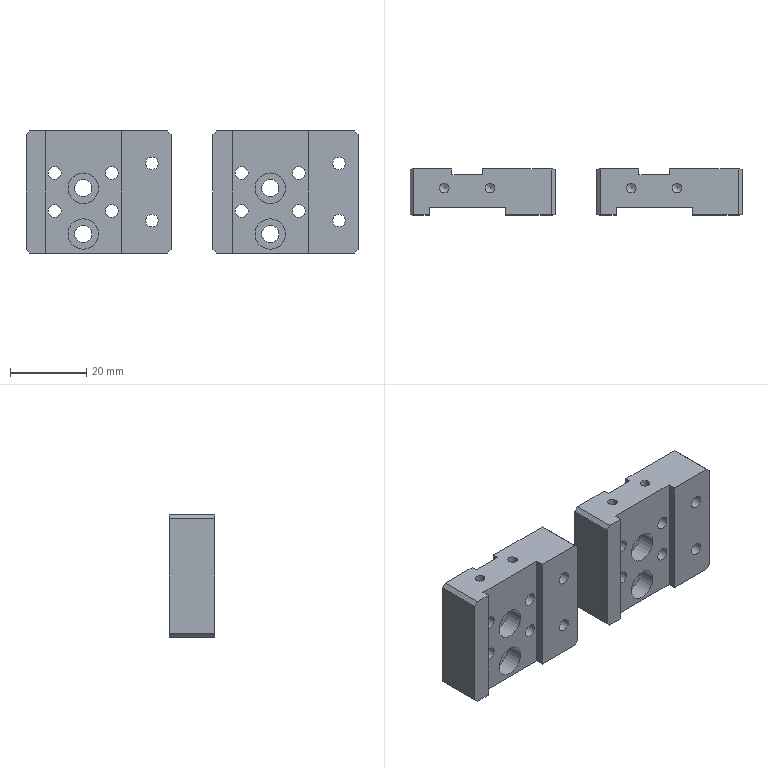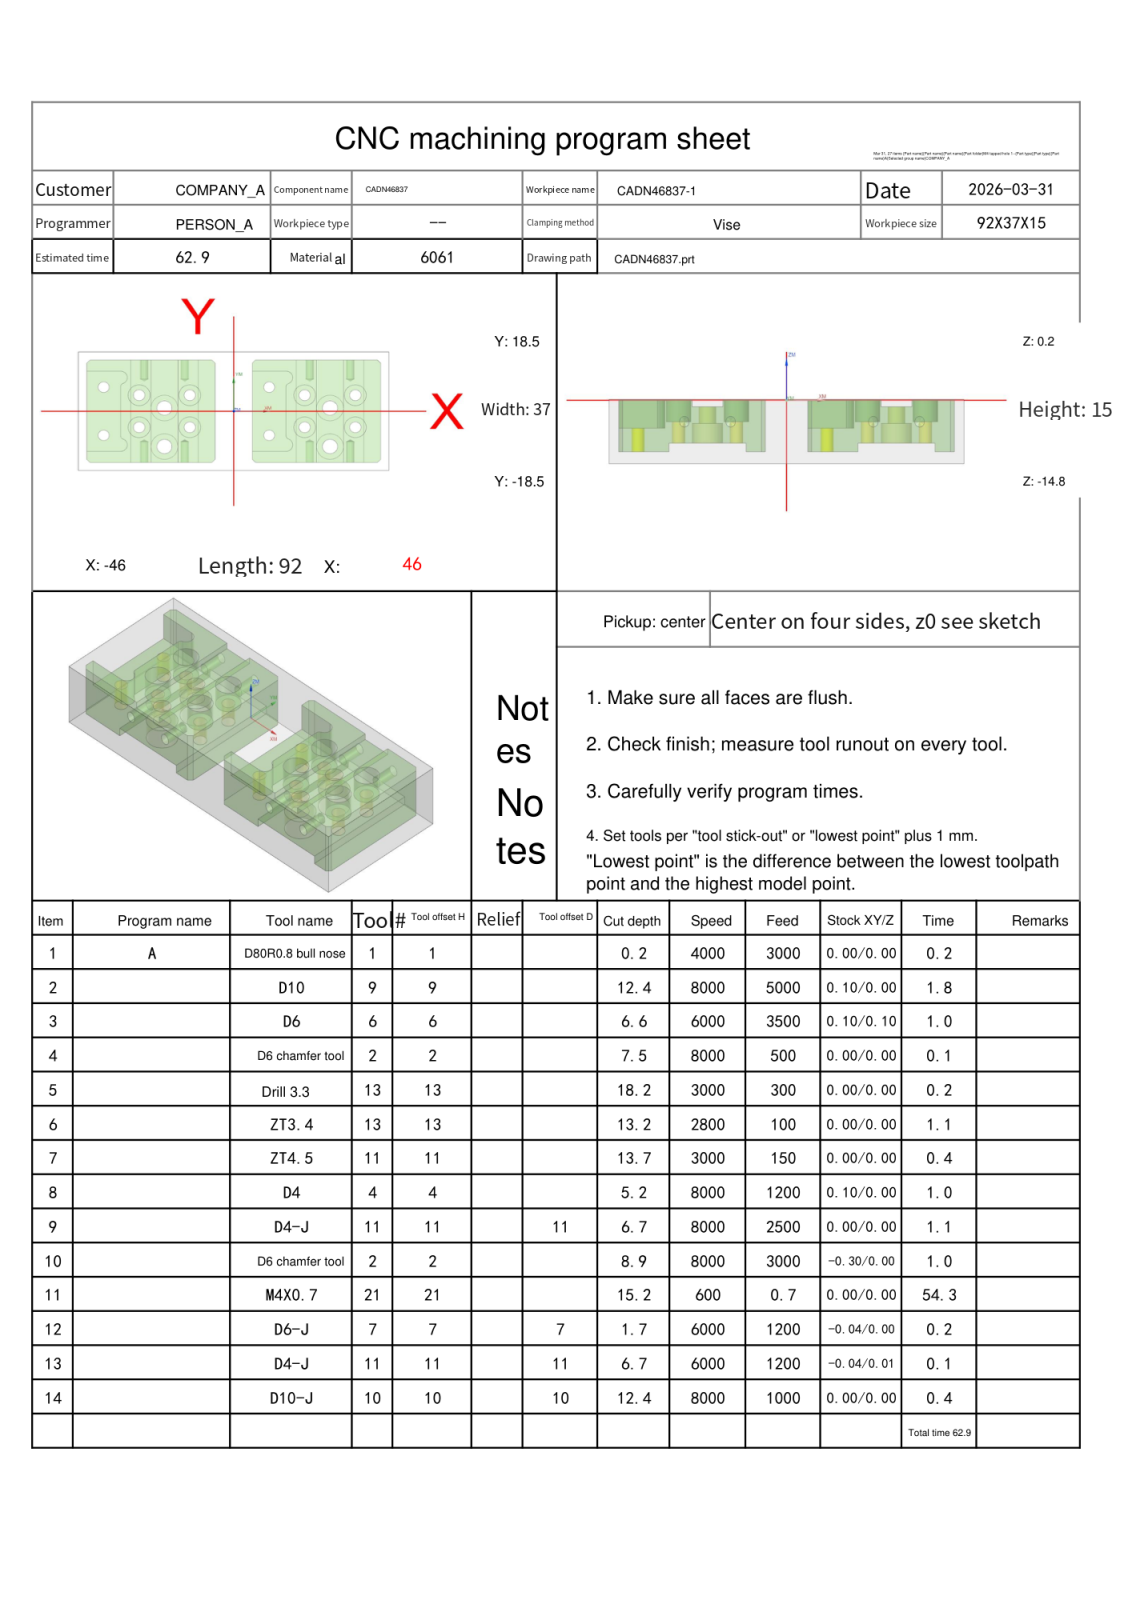NC program | NX | posted by the shop | part box 87 x 12 x 32 mm
Lines 1 to 2025 of 5636, first 1616 of 2023 lines:
%
O0001
(Machine time: 114.10 MIN)
(===Total Tool:10===)
(T1=D80R0.8 bull nose D=80.  R=0.8  D-  H01 Z=0.    )
(T9=D10     D=10.  R=0.   D-  H09 Z=-12.2 )
(T6=D6      D=6.   R=0.   D-  H06 Z=-6.4  )
(T2=D6 chamfer tool   D=6.   R=0.   D-  H02 Z=-8.7  )
(T13=Drill 3.3  D=3.3  DR_a=118 D-  H13 Z=-17.99)
(T11=ZT4.5  D=4.5  DR_a=118 D-  H11 Z=-13.5 )
(T4=D4      D=4.   R=0.   D-  H04 Z=-5.   )
(T21=M4X0.7 D=3.3  DR_a=180 D-  H21 Z=-15.  )
(T7=D6-J    D=6.   R=0.   D7  H07 Z=-1.5  )
(T10=D10-J  D=10.  R=0.   D10 H10 Z=-12.2 )
G80 G90 G17 G49 G40
G91 G28 Z0
M01
N1 T01 M06
(D80R0.8 bull nose  D=80. R=0.8 H=01 ce=0.20 di=0.10)
G00 G90 G54 X-88.5 Y0.0 M03 S4000
G43 H01 Z20.
M08
Z2.1
G01 Z.1 F3000.
X-83.5
X83.5
X88.5
Z2.1
G00 Z20.
G00 G90 X-88.5 Y0.0 M03 S4000
Z20.
Z2.
G01 Z0.0 F1000.
X-83.5
X83.5
X88.5
Z2.
G00 Z20.
G91 G28 Z0.0
M05
M09
G91 G28 Z0.0
M01
N2 T09 M06
(D10  D=10. R=0. H=09 ce=0.10 di=0.00)
G00 G90 G54 X24.5 Y-21.1 M03 S8000
G43 H09 Z20.
M08
Z.5
G01 X6.5 Z.448 F5000.
G02 X2.894 Y-19.606 Z.437 I0.0 J5.1
G01 X1.894 Y-18.606 Z.433
G02 X.4 Y-15. Z.421 I3.606 J3.606
G01 Y15. Z.335
G02 X1.894 Y18.606 Z.323 I5.1 J0.0
G01 X2.894 Y19.606 Z.319
G02 X6.5 Y21.1 Z.308 I3.606 J-3.606
G01 X42.5 Z.204
G02 X46.106 Y19.606 Z.192 I0.0 J-5.1
G01 X47.106 Y18.606 Z.188
G02 X48.6 Y15. Z.177 I-3.606 J-3.606
G01 Y-15. Z.09
G02 X47.106 Y-18.606 Z.079 I-5.1 J0.0
G01 X46.106 Y-19.606 Z.075
G02 X44.375 Y-20.743 Z.069 I-3.606 J3.606
X42.5 Y-21.1 Z.063 I-1.875 J4.743
G01 X6.5 Z-.04
G02 X2.894 Y-19.606 Z-.052 I0.0 J5.1
G01 X1.894 Y-18.606 Z-.056
G02 X.4 Y-15. Z-.067 I3.606 J3.606
G01 Y15. Z-.154
G02 X1.894 Y18.606 Z-.165 I5.1 J0.0
G01 X2.894 Y19.606 Z-.169
G02 X6.5 Y21.1 Z-.181 I3.606 J-3.606
G01 X42.5 Z-.285
G02 X46.106 Y19.606 Z-.296 I0.0 J-5.1
G01 X47.106 Y18.606 Z-.3
G02 X48.6 Y15. Z-.312 I-3.606 J-3.606
G01 Y-15. Z-.398
G02 X47.106 Y-18.606 Z-.41 I-5.1 J0.0
G01 X46.106 Y-19.606 Z-.414
G02 X44.375 Y-20.743 Z-.42 I-3.606 J3.606
X42.5 Y-21.1 Z-.425 I-1.875 J4.743
G01 X6.5 Z-.529
G02 X2.894 Y-19.606 Z-.54 I0.0 J5.1
G01 X1.894 Y-18.606 Z-.544
G02 X.4 Y-15. Z-.556 I3.606 J3.606
G01 Y15. Z-.642
G02 X1.894 Y18.606 Z-.654 I5.1 J0.0
G01 X2.894 Y19.606 Z-.658
G02 X6.5 Y21.1 Z-.669 I3.606 J-3.606
G01 X42.5 Z-.773
G02 X46.106 Y19.606 Z-.784 I0.0 J-5.1
G01 X47.106 Y18.606 Z-.789
G02 X48.6 Y15. Z-.8 I-3.606 J-3.606
G01 Y-15. Z-.886
G02 X47.106 Y-18.606 Z-.898 I-5.1 J0.0
G01 X46.106 Y-19.606 Z-.902
G02 X44.375 Y-20.743 Z-.908 I-3.606 J3.606
X42.5 Y-21.1 Z-.914 I-1.875 J4.743
G01 X6.5 Z-1.017
G02 X2.894 Y-19.606 Z-1.029 I0.0 J5.1
G01 X1.894 Y-18.606 Z-1.033
G02 X.4 Y-15. Z-1.044 I3.606 J3.606
G01 Y15. Z-1.131
G02 X1.894 Y18.606 Z-1.142 I5.1 J0.0
G01 X2.894 Y19.606 Z-1.146
G02 X6.5 Y21.1 Z-1.158 I3.606 J-3.606
G01 X42.5 Z-1.261
G02 X46.106 Y19.606 Z-1.273 I0.0 J-5.1
G01 X47.106 Y18.606 Z-1.277
G02 X48.6 Y15. Z-1.289 I-3.606 J-3.606
G01 Y-15. Z-1.375
G02 X47.106 Y-18.606 Z-1.386 I-5.1 J0.0
G01 X46.106 Y-19.606 Z-1.391
G02 X44.375 Y-20.743 Z-1.397 I-3.606 J3.606
X42.5 Y-21.1 Z-1.402 I-1.875 J4.743
G01 X6.5 Z-1.506
G02 X2.894 Y-19.606 Z-1.517 I0.0 J5.1
G01 X1.894 Y-18.606 Z-1.521
G02 X.4 Y-15. Z-1.533 I3.606 J3.606
G01 Y15. Z-1.619
G02 X1.894 Y18.606 Z-1.631 I5.1 J0.0
G01 X2.894 Y19.606 Z-1.635
G02 X6.5 Y21.1 Z-1.646 I3.606 J-3.606
G01 X42.5 Z-1.75
G02 X46.106 Y19.606 Z-1.761 I0.0 J-5.1
G01 X47.106 Y18.606 Z-1.765
G02 X48.6 Y15. Z-1.777 I-3.606 J-3.606
G01 Y-15. Z-1.863
G02 X47.106 Y-18.606 Z-1.875 I-5.1 J0.0
G01 X46.106 Y-19.606 Z-1.879
G02 X44.375 Y-20.743 Z-1.885 I-3.606 J3.606
X42.5 Y-21.1 Z-1.89 I-1.875 J4.743
G01 X6.5 Z-1.994
G02 X2.894 Y-19.606 Z-2.006 I0.0 J5.1
G01 X1.894 Y-18.606 Z-2.01
G02 X.4 Y-15. Z-2.021 I3.606 J3.606
G01 Y15. Z-2.108
G02 X1.894 Y18.606 Z-2.119 I5.1 J0.0
G01 X2.894 Y19.606 Z-2.123
G02 X6.5 Y21.1 Z-2.135 I3.606 J-3.606
G01 X42.5 Z-2.238
G02 X46.106 Y19.606 Z-2.25 I0.0 J-5.1
G01 X47.106 Y18.606 Z-2.254
G02 X48.6 Y15. Z-2.265 I-3.606 J-3.606
G01 Y-15. Z-2.352
G02 X47.106 Y-18.606 Z-2.363 I-5.1 J0.0
G01 X46.106 Y-19.606 Z-2.367
G02 X44.375 Y-20.743 Z-2.373 I-3.606 J3.606
X42.5 Y-21.1 Z-2.379 I-1.875 J4.743
G01 X6.5 Z-2.483
G02 X2.894 Y-19.606 Z-2.494 I0.0 J5.1
G01 X1.894 Y-18.606 Z-2.498
G02 X.4 Y-15. Z-2.51 I3.606 J3.606
G01 Y15. Z-2.596
G02 X1.894 Y18.606 Z-2.608 I5.1 J0.0
G01 X2.894 Y19.606 Z-2.612
G02 X6.5 Y21.1 Z-2.623 I3.606 J-3.606
G01 X42.5 Z-2.727
G02 X46.106 Y19.606 Z-2.738 I0.0 J-5.1
G01 X47.106 Y18.606 Z-2.742
G02 X48.6 Y15. Z-2.754 I-3.606 J-3.606
G01 Y-15. Z-2.84
G02 X47.106 Y-18.606 Z-2.852 I-5.1 J0.0
G01 X46.106 Y-19.606 Z-2.856
G02 X44.375 Y-20.743 Z-2.862 I-3.606 J3.606
X42.5 Y-21.1 Z-2.867 I-1.875 J4.743
G01 X6.5 Z-2.971
G02 X2.894 Y-19.606 Z-2.983 I0.0 J5.1
G01 X1.894 Y-18.606 Z-2.987
G02 X.4 Y-15. Z-2.998 I3.606 J3.606
G01 Y15. Z-3.085
G02 X1.894 Y18.606 Z-3.096 I5.1 J0.0
G01 X2.894 Y19.606 Z-3.1
G02 X6.5 Y21.1 Z-3.112 I3.606 J-3.606
G01 X42.5 Z-3.215
G02 X46.106 Y19.606 Z-3.227 I0.0 J-5.1
G01 X47.106 Y18.606 Z-3.231
G02 X48.6 Y15. Z-3.242 I-3.606 J-3.606
G01 Y-15. Z-3.329
G02 X47.106 Y-18.606 Z-3.34 I-5.1 J0.0
G01 X46.106 Y-19.606 Z-3.344
G02 X44.375 Y-20.743 Z-3.35 I-3.606 J3.606
X42.5 Y-21.1 Z-3.356 I-1.875 J4.743
G01 X6.5 Z-3.46
G02 X2.894 Y-19.606 Z-3.471 I0.0 J5.1
G01 X1.894 Y-18.606 Z-3.475
G02 X.4 Y-15. Z-3.487 I3.606 J3.606
G01 Y15. Z-3.573
G02 X1.894 Y18.606 Z-3.585 I5.1 J0.0
G01 X2.894 Y19.606 Z-3.589
G02 X6.5 Y21.1 Z-3.6 I3.606 J-3.606
G01 X42.5 Z-3.704
G02 X46.106 Y19.606 Z-3.715 I0.0 J-5.1
G01 X47.106 Y18.606 Z-3.719
G02 X48.6 Y15. Z-3.731 I-3.606 J-3.606
G01 Y-15. Z-3.817
G02 X47.106 Y-18.606 Z-3.829 I-5.1 J0.0
G01 X46.106 Y-19.606 Z-3.833
G02 X44.375 Y-20.743 Z-3.839 I-3.606 J3.606
X42.5 Y-21.1 Z-3.844 I-1.875 J4.743
G01 X6.5 Z-3.948
G02 X2.894 Y-19.606 Z-3.959 I0.0 J5.1
G01 X1.894 Y-18.606 Z-3.964
G02 X.4 Y-15. Z-3.975 I3.606 J3.606
G01 Y15. Z-4.061
G02 X1.894 Y18.606 Z-4.073 I5.1 J0.0
G01 X2.894 Y19.606 Z-4.077
G02 X6.5 Y21.1 Z-4.089 I3.606 J-3.606
G01 X42.5 Z-4.192
G02 X46.106 Y19.606 Z-4.204 I0.0 J-5.1
G01 X47.106 Y18.606 Z-4.208
G02 X48.6 Y15. Z-4.219 I-3.606 J-3.606
G01 Y-15. Z-4.306
G02 X47.106 Y-18.606 Z-4.317 I-5.1 J0.0
G01 X46.106 Y-19.606 Z-4.321
G02 X44.375 Y-20.743 Z-4.327 I-3.606 J3.606
X42.5 Y-21.1 Z-4.333 I-1.875 J4.743
G01 X6.5 Z-4.436
G02 X2.894 Y-19.606 Z-4.448 I0.0 J5.1
G01 X1.894 Y-18.606 Z-4.452
G02 X.4 Y-15. Z-4.464 I3.606 J3.606
G01 Y15. Z-4.55
G02 X1.894 Y18.606 Z-4.561 I5.1 J0.0
G01 X2.894 Y19.606 Z-4.566
G02 X6.5 Y21.1 Z-4.577 I3.606 J-3.606
G01 X42.5 Z-4.681
G02 X46.106 Y19.606 Z-4.692 I0.0 J-5.1
G01 X47.106 Y18.606 Z-4.696
G02 X48.6 Y15. Z-4.708 I-3.606 J-3.606
G01 Y-15. Z-4.794
G02 X47.106 Y-18.606 Z-4.806 I-5.1 J0.0
G01 X46.106 Y-19.606 Z-4.81
G02 X44.375 Y-20.743 Z-4.816 I-3.606 J3.606
X42.5 Y-21.1 Z-4.821 I-1.875 J4.743
G01 X6.5 Z-4.925
G02 X2.894 Y-19.606 Z-4.936 I0.0 J5.1
G01 X1.894 Y-18.606 Z-4.94
G02 X.4 Y-15. Z-4.952 I3.606 J3.606
G01 Y15. Z-5.038
G02 X1.894 Y18.606 Z-5.05 I5.1 J0.0
G01 X2.894 Y19.606 Z-5.054
G02 X6.5 Y21.1 Z-5.065 I3.606 J-3.606
G01 X42.5 Z-5.169
G02 X46.106 Y19.606 Z-5.181 I0.0 J-5.1
G01 X47.106 Y18.606 Z-5.185
G02 X48.6 Y15. Z-5.196 I-3.606 J-3.606
G01 Y-15. Z-5.283
G02 X47.106 Y-18.606 Z-5.294 I-5.1 J0.0
G01 X46.106 Y-19.606 Z-5.298
G02 X44.375 Y-20.743 Z-5.304 I-3.606 J3.606
X42.5 Y-21.1 Z-5.31 I-1.875 J4.743
G01 X6.5 Z-5.413
G02 X2.894 Y-19.606 Z-5.425 I0.0 J5.1
G01 X1.894 Y-18.606 Z-5.429
G02 X.4 Y-15. Z-5.44 I3.606 J3.606
G01 Y15. Z-5.527
G02 X1.894 Y18.606 Z-5.538 I5.1 J0.0
G01 X2.894 Y19.606 Z-5.542
G02 X6.5 Y21.1 Z-5.554 I3.606 J-3.606
G01 X42.5 Z-5.658
G02 X46.106 Y19.606 Z-5.669 I0.0 J-5.1
G01 X47.106 Y18.606 Z-5.673
G02 X48.6 Y15. Z-5.685 I-3.606 J-3.606
G01 Y-15. Z-5.771
G02 X47.106 Y-18.606 Z-5.783 I-5.1 J0.0
G01 X46.106 Y-19.606 Z-5.787
G02 X44.375 Y-20.743 Z-5.793 I-3.606 J3.606
X42.5 Y-21.1 Z-5.798 I-1.875 J4.743
G01 X6.5 Z-5.902
G02 X2.894 Y-19.606 Z-5.913 I0.0 J5.1
G01 X1.894 Y-18.606 Z-5.917
G02 X.4 Y-15. Z-5.929 I3.606 J3.606
G01 Y15. Z-6.015
G02 X1.894 Y18.606 Z-6.027 I5.1 J0.0
G01 X2.894 Y19.606 Z-6.031
G02 X6.5 Y21.1 Z-6.042 I3.606 J-3.606
G01 X42.5 Z-6.146
G02 X46.106 Y19.606 Z-6.158 I0.0 J-5.1
G01 X47.106 Y18.606 Z-6.162
G02 X48.6 Y15. Z-6.173 I-3.606 J-3.606
G01 Y-15. Z-6.26
G02 X47.106 Y-18.606 Z-6.271 I-5.1 J0.0
G01 X46.106 Y-19.606 Z-6.275
G02 X44.375 Y-20.743 Z-6.281 I-3.606 J3.606
X42.5 Y-21.1 Z-6.287 I-1.875 J4.743
G01 X6.5 Z-6.39
G02 X2.894 Y-19.606 Z-6.402 I0.0 J5.1
G01 X1.894 Y-18.606 Z-6.406
G02 X.4 Y-15. Z-6.417 I3.606 J3.606
G01 Y15. Z-6.504
G02 X1.894 Y18.606 Z-6.515 I5.1 J0.0
G01 X2.894 Y19.606 Z-6.519
G02 X6.5 Y21.1 Z-6.531 I3.606 J-3.606
G01 X42.5 Z-6.635
G02 X46.106 Y19.606 Z-6.646 I0.0 J-5.1
G01 X47.106 Y18.606 Z-6.65
G02 X48.6 Y15. Z-6.662 I-3.606 J-3.606
G01 Y-15. Z-6.748
G02 X47.106 Y-18.606 Z-6.76 I-5.1 J0.0
G01 X46.106 Y-19.606 Z-6.764
G02 X44.375 Y-20.743 Z-6.77 I-3.606 J3.606
X42.5 Y-21.1 Z-6.775 I-1.875 J4.743
G01 X6.5 Z-6.879
G02 X2.894 Y-19.606 Z-6.89 I0.0 J5.1
G01 X1.894 Y-18.606 Z-6.894
G02 X.4 Y-15. Z-6.906 I3.606 J3.606
G01 Y15. Z-6.992
G02 X1.894 Y18.606 Z-7.004 I5.1 J0.0
G01 X2.894 Y19.606 Z-7.008
G02 X6.5 Y21.1 Z-7.019 I3.606 J-3.606
G01 X42.5 Z-7.123
G02 X46.106 Y19.606 Z-7.134 I0.0 J-5.1
G01 X47.106 Y18.606 Z-7.139
G02 X48.6 Y15. Z-7.15 I-3.606 J-3.606
G01 Y-15. Z-7.236
G02 X47.106 Y-18.606 Z-7.248 I-5.1 J0.0
G01 X46.106 Y-19.606 Z-7.252
G02 X44.375 Y-20.743 Z-7.258 I-3.606 J3.606
X42.5 Y-21.1 Z-7.264 I-1.875 J4.743
G01 X6.5 Z-7.367
G02 X2.894 Y-19.606 Z-7.379 I0.0 J5.1
G01 X1.894 Y-18.606 Z-7.383
G02 X.4 Y-15. Z-7.394 I3.606 J3.606
G01 Y15. Z-7.481
G02 X1.894 Y18.606 Z-7.492 I5.1 J0.0
G01 X2.894 Y19.606 Z-7.496
G02 X6.5 Y21.1 Z-7.508 I3.606 J-3.606
G01 X42.5 Z-7.611
G02 X46.106 Y19.606 Z-7.623 I0.0 J-5.1
G01 X47.106 Y18.606 Z-7.627
G02 X48.6 Y15. Z-7.639 I-3.606 J-3.606
G01 Y-15. Z-7.725
G02 X47.106 Y-18.606 Z-7.736 I-5.1 J0.0
G01 X46.106 Y-19.606 Z-7.741
G02 X44.375 Y-20.743 Z-7.747 I-3.606 J3.606
X42.5 Y-21.1 Z-7.752 I-1.875 J4.743
G01 X6.5 Z-7.856
G02 X2.894 Y-19.606 Z-7.867 I0.0 J5.1
G01 X1.894 Y-18.606 Z-7.871
G02 X.4 Y-15. Z-7.883 I3.606 J3.606
G01 Y15. Z-7.969
G02 X1.894 Y18.606 Z-7.981 I5.1 J0.0
G01 X2.894 Y19.606 Z-7.985
G02 X6.5 Y21.1 Z-7.996 I3.606 J-3.606
G01 X42.5 Z-8.1
G02 X46.106 Y19.606 Z-8.111 I0.0 J-5.1
G01 X47.106 Y18.606 Z-8.115
G02 X48.6 Y15. Z-8.127 I-3.606 J-3.606
G01 Y-15. Z-8.213
G02 X47.106 Y-18.606 Z-8.225 I-5.1 J0.0
G01 X46.106 Y-19.606 Z-8.229
G02 X44.375 Y-20.743 Z-8.235 I-3.606 J3.606
X42.5 Y-21.1 Z-8.24 I-1.875 J4.743
G01 X6.5 Z-8.344
G02 X2.894 Y-19.606 Z-8.356 I0.0 J5.1
G01 X1.894 Y-18.606 Z-8.36
G02 X.4 Y-15. Z-8.371 I3.606 J3.606
G01 Y15. Z-8.458
G02 X1.894 Y18.606 Z-8.469 I5.1 J0.0
G01 X2.894 Y19.606 Z-8.473
G02 X6.5 Y21.1 Z-8.485 I3.606 J-3.606
G01 X42.5 Z-8.588
G02 X46.106 Y19.606 Z-8.6 I0.0 J-5.1
G01 X47.106 Y18.606 Z-8.604
G02 X48.6 Y15. Z-8.615 I-3.606 J-3.606
G01 Y-15. Z-8.702
G02 X47.106 Y-18.606 Z-8.713 I-5.1 J0.0
G01 X46.106 Y-19.606 Z-8.717
G02 X44.375 Y-20.743 Z-8.723 I-3.606 J3.606
X42.5 Y-21.1 Z-8.729 I-1.875 J4.743
G01 X6.5 Z-8.833
G02 X2.894 Y-19.606 Z-8.844 I0.0 J5.1
G01 X1.894 Y-18.606 Z-8.848
G02 X.4 Y-15. Z-8.86 I3.606 J3.606
G01 Y15. Z-8.946
G02 X1.894 Y18.606 Z-8.958 I5.1 J0.0
G01 X2.894 Y19.606 Z-8.962
G02 X6.5 Y21.1 Z-8.973 I3.606 J-3.606
G01 X42.5 Z-9.077
G02 X46.106 Y19.606 Z-9.088 I0.0 J-5.1
G01 X47.106 Y18.606 Z-9.092
G02 X48.6 Y15. Z-9.104 I-3.606 J-3.606
G01 Y-15. Z-9.19
G02 X47.106 Y-18.606 Z-9.202 I-5.1 J0.0
G01 X46.106 Y-19.606 Z-9.206
G02 X44.375 Y-20.743 Z-9.212 I-3.606 J3.606
X42.5 Y-21.1 Z-9.217 I-1.875 J4.743
G01 X6.5 Z-9.321
G02 X2.894 Y-19.606 Z-9.333 I0.0 J5.1
G01 X1.894 Y-18.606 Z-9.337
G02 X.4 Y-15. Z-9.348 I3.606 J3.606
G01 Y15. Z-9.435
G02 X1.894 Y18.606 Z-9.446 I5.1 J0.0
G01 X2.894 Y19.606 Z-9.45
G02 X6.5 Y21.1 Z-9.462 I3.606 J-3.606
G01 X42.5 Z-9.565
G02 X46.106 Y19.606 Z-9.577 I0.0 J-5.1
G01 X47.106 Y18.606 Z-9.581
G02 X48.6 Y15. Z-9.592 I-3.606 J-3.606
G01 Y-15. Z-9.679
G02 X47.106 Y-18.606 Z-9.69 I-5.1 J0.0
G01 X46.106 Y-19.606 Z-9.694
G02 X44.375 Y-20.743 Z-9.7 I-3.606 J3.606
X42.5 Y-21.1 Z-9.706 I-1.875 J4.743
G01 X6.5 Z-9.81
G02 X2.894 Y-19.606 Z-9.821 I0.0 J5.1
G01 X1.894 Y-18.606 Z-9.825
G02 X.4 Y-15. Z-9.837 I3.606 J3.606
G01 Y15. Z-9.923
G02 X1.894 Y18.606 Z-9.935 I5.1 J0.0
G01 X2.894 Y19.606 Z-9.939
G02 X6.5 Y21.1 Z-9.95 I3.606 J-3.606
G01 X42.5 Z-10.054
G02 X46.106 Y19.606 Z-10.065 I0.0 J-5.1
G01 X47.106 Y18.606 Z-10.069
G02 X48.6 Y15. Z-10.081 I-3.606 J-3.606
G01 Y-15. Z-10.167
G02 X47.106 Y-18.606 Z-10.179 I-5.1 J0.0
G01 X46.106 Y-19.606 Z-10.183
G02 X44.375 Y-20.743 Z-10.189 I-3.606 J3.606
X42.5 Y-21.1 Z-10.194 I-1.875 J4.743
G01 X6.5 Z-10.298
G02 X2.894 Y-19.606 Z-10.309 I0.0 J5.1
G01 X1.894 Y-18.606 Z-10.314
G02 X.4 Y-15. Z-10.325 I3.606 J3.606
G01 Y15. Z-10.411
G02 X1.894 Y18.606 Z-10.423 I5.1 J0.0
G01 X2.894 Y19.606 Z-10.427
G02 X6.5 Y21.1 Z-10.439 I3.606 J-3.606
G01 X42.5 Z-10.542
G02 X46.106 Y19.606 Z-10.554 I0.0 J-5.1
G01 X47.106 Y18.606 Z-10.558
G02 X48.6 Y15. Z-10.569 I-3.606 J-3.606
G01 Y-15. Z-10.656
G02 X47.106 Y-18.606 Z-10.667 I-5.1 J0.0
G01 X46.106 Y-19.606 Z-10.671
G02 X44.375 Y-20.743 Z-10.677 I-3.606 J3.606
X42.5 Y-21.1 Z-10.683 I-1.875 J4.743
G01 X6.5 Z-10.786
G02 X2.894 Y-19.606 Z-10.798 I0.0 J5.1
G01 X1.894 Y-18.606 Z-10.802
G02 X.4 Y-15. Z-10.814 I3.606 J3.606
G01 Y15. Z-10.9
G02 X1.894 Y18.606 Z-10.911 I5.1 J0.0
G01 X2.894 Y19.606 Z-10.916
G02 X6.5 Y21.1 Z-10.927 I3.606 J-3.606
G01 X42.5 Z-11.031
G02 X46.106 Y19.606 Z-11.042 I0.0 J-5.1
G01 X47.106 Y18.606 Z-11.046
G02 X48.6 Y15. Z-11.058 I-3.606 J-3.606
G01 Y-15. Z-11.144
G02 X47.106 Y-18.606 Z-11.156 I-5.1 J0.0
G01 X46.106 Y-19.606 Z-11.16
G02 X44.375 Y-20.743 Z-11.166 I-3.606 J3.606
X42.5 Y-21.1 Z-11.171 I-1.875 J4.743
G01 X6.5 Z-11.275
G02 X2.894 Y-19.606 Z-11.286 I0.0 J5.1
G01 X1.894 Y-18.606 Z-11.29
G02 X.4 Y-15. Z-11.302 I3.606 J3.606
G01 Y15. Z-11.388
G02 X1.894 Y18.606 Z-11.4 I5.1 J0.0
G01 X2.894 Y19.606 Z-11.404
G02 X6.5 Y21.1 Z-11.415 I3.606 J-3.606
G01 X42.5 Z-11.519
G02 X46.106 Y19.606 Z-11.531 I0.0 J-5.1
G01 X47.106 Y18.606 Z-11.535
G02 X48.6 Y15. Z-11.546 I-3.606 J-3.606
G01 Y-15. Z-11.633
G02 X47.106 Y-18.606 Z-11.644 I-5.1 J0.0
G01 X46.106 Y-19.606 Z-11.648
G02 X44.375 Y-20.743 Z-11.654 I-3.606 J3.606
X42.5 Y-21.1 Z-11.66 I-1.875 J4.743
G01 X6.5 Z-11.763
G02 X2.894 Y-19.606 Z-11.775 I0.0 J5.1
G01 X1.894 Y-18.606 Z-11.779
G02 X.4 Y-15. Z-11.79 I3.606 J3.606
G01 Y15. Z-11.877
G02 X1.894 Y18.606 Z-11.888 I5.1 J0.0
G01 X2.894 Y19.606 Z-11.892
G02 X6.5 Y21.1 Z-11.904 I3.606 J-3.606
G01 X42.5 Z-12.008
G02 X46.106 Y19.606 Z-12.019 I0.0 J-5.1
G01 X47.106 Y18.606 Z-12.023
G02 X48.6 Y15. Z-12.035 I-3.606 J-3.606
G01 Y-15. Z-12.121
G02 X47.106 Y-18.606 Z-12.133 I-5.1 J0.0
G01 X46.106 Y-19.606 Z-12.137
G02 X44.375 Y-20.743 Z-12.143 I-3.606 J3.606
X42.5 Y-21.1 Z-12.148 I-1.875 J4.743
G01 X24.5 Z-12.2
X6.5
G02 X2.894 Y-19.606 I0.0 J5.1
G01 X1.894 Y-18.606
G02 X.4 Y-15. I3.606 J3.606
G01 Y15.
G02 X1.894 Y18.606 I5.1 J0.0
G01 X2.894 Y19.606
G02 X6.5 Y21.1 I3.606 J-3.606
G01 X42.5
G02 X46.106 Y19.606 I0.0 J-5.1
G01 X47.106 Y18.606
G02 X48.6 Y15. I-3.606 J-3.606
G01 Y-15.
G02 X47.106 Y-18.606 I-5.1 J0.0
G01 X46.106 Y-19.606
G02 X42.5 Y-21.1 I-3.606 J3.606
G01 X24.5
X24.
Z-11.2
G00 Z20.
X-24.5
Z.5
G01 X-42.5 Z.448
G02 X-46.106 Y-19.606 Z.437 I0.0 J5.1
G01 X-47.106 Y-18.606 Z.433
G02 X-48.6 Y-15. Z.421 I3.606 J3.606
G01 Y15. Z.335
G02 X-47.106 Y18.606 Z.323 I5.1 J0.0
G01 X-46.106 Y19.606 Z.319
G02 X-42.5 Y21.1 Z.308 I3.606 J-3.606
G01 X-6.5 Z.204
G02 X-2.894 Y19.606 Z.192 I0.0 J-5.1
G01 X-1.894 Y18.606 Z.188
G02 X-.4 Y15. Z.177 I-3.606 J-3.606
G01 Y-15. Z.09
G02 X-1.894 Y-18.606 Z.079 I-5.1 J0.0
G01 X-2.894 Y-19.606 Z.075
G02 X-6.5 Y-21.1 Z.063 I-3.606 J3.606
G01 X-42.5 Z-.04
G02 X-46.106 Y-19.606 Z-.052 I0.0 J5.1
G01 X-47.106 Y-18.606 Z-.056
G02 X-48.6 Y-15. Z-.067 I3.606 J3.606
G01 Y15. Z-.154
G02 X-47.106 Y18.606 Z-.165 I5.1 J0.0
G01 X-46.106 Y19.606 Z-.169
G02 X-42.5 Y21.1 Z-.181 I3.606 J-3.606
G01 X-6.5 Z-.285
G02 X-2.894 Y19.606 Z-.296 I0.0 J-5.1
G01 X-1.894 Y18.606 Z-.3
G02 X-.4 Y15. Z-.312 I-3.606 J-3.606
G01 Y-15. Z-.398
G02 X-1.894 Y-18.606 Z-.41 I-5.1 J0.0
G01 X-2.894 Y-19.606 Z-.414
G02 X-6.5 Y-21.1 Z-.425 I-3.606 J3.606
G01 X-42.5 Z-.529
G02 X-46.106 Y-19.606 Z-.54 I0.0 J5.1
G01 X-47.106 Y-18.606 Z-.544
G02 X-48.6 Y-15. Z-.556 I3.606 J3.606
G01 Y15. Z-.642
G02 X-47.106 Y18.606 Z-.654 I5.1 J0.0
G01 X-46.106 Y19.606 Z-.658
G02 X-42.5 Y21.1 Z-.669 I3.606 J-3.606
G01 X-6.5 Z-.773
G02 X-2.894 Y19.606 Z-.784 I0.0 J-5.1
G01 X-1.894 Y18.606 Z-.789
G02 X-.4 Y15. Z-.8 I-3.606 J-3.606
G01 Y-15. Z-.886
G02 X-1.894 Y-18.606 Z-.898 I-5.1 J0.0
G01 X-2.894 Y-19.606 Z-.902
G02 X-6.5 Y-21.1 Z-.914 I-3.606 J3.606
G01 X-42.5 Z-1.017
G02 X-46.106 Y-19.606 Z-1.029 I0.0 J5.1
G01 X-47.106 Y-18.606 Z-1.033
G02 X-48.6 Y-15. Z-1.044 I3.606 J3.606
G01 Y15. Z-1.131
G02 X-47.106 Y18.606 Z-1.142 I5.1 J0.0
G01 X-46.106 Y19.606 Z-1.146
G02 X-42.5 Y21.1 Z-1.158 I3.606 J-3.606
G01 X-6.5 Z-1.261
G02 X-2.894 Y19.606 Z-1.273 I0.0 J-5.1
G01 X-1.894 Y18.606 Z-1.277
G02 X-.4 Y15. Z-1.289 I-3.606 J-3.606
G01 Y-15. Z-1.375
G02 X-1.894 Y-18.606 Z-1.386 I-5.1 J0.0
G01 X-2.894 Y-19.606 Z-1.391
G02 X-6.5 Y-21.1 Z-1.402 I-3.606 J3.606
G01 X-42.5 Z-1.506
G02 X-46.106 Y-19.606 Z-1.517 I0.0 J5.1
G01 X-47.106 Y-18.606 Z-1.521
G02 X-48.6 Y-15. Z-1.533 I3.606 J3.606
G01 Y15. Z-1.619
G02 X-47.106 Y18.606 Z-1.631 I5.1 J0.0
G01 X-46.106 Y19.606 Z-1.635
G02 X-42.5 Y21.1 Z-1.646 I3.606 J-3.606
G01 X-6.5 Z-1.75
G02 X-2.894 Y19.606 Z-1.761 I0.0 J-5.1
G01 X-1.894 Y18.606 Z-1.765
G02 X-.4 Y15. Z-1.777 I-3.606 J-3.606
G01 Y-15. Z-1.863
G02 X-1.894 Y-18.606 Z-1.875 I-5.1 J0.0
G01 X-2.894 Y-19.606 Z-1.879
G02 X-6.5 Y-21.1 Z-1.89 I-3.606 J3.606
G01 X-42.5 Z-1.994
G02 X-46.106 Y-19.606 Z-2.006 I0.0 J5.1
G01 X-47.106 Y-18.606 Z-2.01
G02 X-48.6 Y-15. Z-2.021 I3.606 J3.606
G01 Y15. Z-2.108
G02 X-47.106 Y18.606 Z-2.119 I5.1 J0.0
G01 X-46.106 Y19.606 Z-2.123
G02 X-42.5 Y21.1 Z-2.135 I3.606 J-3.606
G01 X-6.5 Z-2.238
G02 X-2.894 Y19.606 Z-2.25 I0.0 J-5.1
G01 X-1.894 Y18.606 Z-2.254
G02 X-.4 Y15. Z-2.265 I-3.606 J-3.606
G01 Y-15. Z-2.352
G02 X-1.894 Y-18.606 Z-2.363 I-5.1 J0.0
G01 X-2.894 Y-19.606 Z-2.367
G02 X-6.5 Y-21.1 Z-2.379 I-3.606 J3.606
G01 X-42.5 Z-2.483
G02 X-46.106 Y-19.606 Z-2.494 I0.0 J5.1
G01 X-47.106 Y-18.606 Z-2.498
G02 X-48.6 Y-15. Z-2.51 I3.606 J3.606
G01 Y15. Z-2.596
G02 X-47.106 Y18.606 Z-2.608 I5.1 J0.0
G01 X-46.106 Y19.606 Z-2.612
G02 X-42.5 Y21.1 Z-2.623 I3.606 J-3.606
G01 X-6.5 Z-2.727
G02 X-2.894 Y19.606 Z-2.738 I0.0 J-5.1
G01 X-1.894 Y18.606 Z-2.742
G02 X-.4 Y15. Z-2.754 I-3.606 J-3.606
G01 Y-15. Z-2.84
G02 X-1.894 Y-18.606 Z-2.852 I-5.1 J0.0
G01 X-2.894 Y-19.606 Z-2.856
G02 X-6.5 Y-21.1 Z-2.867 I-3.606 J3.606
G01 X-42.5 Z-2.971
G02 X-46.106 Y-19.606 Z-2.983 I0.0 J5.1
G01 X-47.106 Y-18.606 Z-2.987
G02 X-48.6 Y-15. Z-2.998 I3.606 J3.606
G01 Y15. Z-3.085
G02 X-47.106 Y18.606 Z-3.096 I5.1 J0.0
G01 X-46.106 Y19.606 Z-3.1
G02 X-42.5 Y21.1 Z-3.112 I3.606 J-3.606
G01 X-6.5 Z-3.215
G02 X-2.894 Y19.606 Z-3.227 I0.0 J-5.1
G01 X-1.894 Y18.606 Z-3.231
G02 X-.4 Y15. Z-3.242 I-3.606 J-3.606
G01 Y-15. Z-3.329
G02 X-1.894 Y-18.606 Z-3.34 I-5.1 J0.0
G01 X-2.894 Y-19.606 Z-3.344
G02 X-6.5 Y-21.1 Z-3.356 I-3.606 J3.606
G01 X-42.5 Z-3.46
G02 X-46.106 Y-19.606 Z-3.471 I0.0 J5.1
G01 X-47.106 Y-18.606 Z-3.475
G02 X-48.6 Y-15. Z-3.487 I3.606 J3.606
G01 Y15. Z-3.573
G02 X-47.106 Y18.606 Z-3.585 I5.1 J0.0
G01 X-46.106 Y19.606 Z-3.589
G02 X-42.5 Y21.1 Z-3.6 I3.606 J-3.606
G01 X-6.5 Z-3.704
G02 X-2.894 Y19.606 Z-3.715 I0.0 J-5.1
G01 X-1.894 Y18.606 Z-3.719
G02 X-.4 Y15. Z-3.731 I-3.606 J-3.606
G01 Y-15. Z-3.817
G02 X-1.894 Y-18.606 Z-3.829 I-5.1 J0.0
G01 X-2.894 Y-19.606 Z-3.833
G02 X-6.5 Y-21.1 Z-3.844 I-3.606 J3.606
G01 X-42.5 Z-3.948
G02 X-46.106 Y-19.606 Z-3.959 I0.0 J5.1
G01 X-47.106 Y-18.606 Z-3.964
G02 X-48.6 Y-15. Z-3.975 I3.606 J3.606
G01 Y15. Z-4.061
G02 X-47.106 Y18.606 Z-4.073 I5.1 J0.0
G01 X-46.106 Y19.606 Z-4.077
G02 X-42.5 Y21.1 Z-4.089 I3.606 J-3.606
G01 X-6.5 Z-4.192
G02 X-2.894 Y19.606 Z-4.204 I0.0 J-5.1
G01 X-1.894 Y18.606 Z-4.208
G02 X-.4 Y15. Z-4.219 I-3.606 J-3.606
G01 Y-15. Z-4.306
G02 X-1.894 Y-18.606 Z-4.317 I-5.1 J0.0
G01 X-2.894 Y-19.606 Z-4.321
G02 X-6.5 Y-21.1 Z-4.333 I-3.606 J3.606
G01 X-42.5 Z-4.436
G02 X-46.106 Y-19.606 Z-4.448 I0.0 J5.1
G01 X-47.106 Y-18.606 Z-4.452
G02 X-48.6 Y-15. Z-4.464 I3.606 J3.606
G01 Y15. Z-4.55
G02 X-47.106 Y18.606 Z-4.561 I5.1 J0.0
G01 X-46.106 Y19.606 Z-4.566
G02 X-42.5 Y21.1 Z-4.577 I3.606 J-3.606
G01 X-6.5 Z-4.681
G02 X-2.894 Y19.606 Z-4.692 I0.0 J-5.1
G01 X-1.894 Y18.606 Z-4.696
G02 X-.4 Y15. Z-4.708 I-3.606 J-3.606
G01 Y-15. Z-4.794
G02 X-1.894 Y-18.606 Z-4.806 I-5.1 J0.0
G01 X-2.894 Y-19.606 Z-4.81
G02 X-6.5 Y-21.1 Z-4.821 I-3.606 J3.606
G01 X-42.5 Z-4.925
G02 X-46.106 Y-19.606 Z-4.936 I0.0 J5.1
G01 X-47.106 Y-18.606 Z-4.94
G02 X-48.6 Y-15. Z-4.952 I3.606 J3.606
G01 Y15. Z-5.038
G02 X-47.106 Y18.606 Z-5.05 I5.1 J0.0
G01 X-46.106 Y19.606 Z-5.054
G02 X-42.5 Y21.1 Z-5.065 I3.606 J-3.606
G01 X-6.5 Z-5.169
G02 X-2.894 Y19.606 Z-5.181 I0.0 J-5.1
G01 X-1.894 Y18.606 Z-5.185
G02 X-.4 Y15. Z-5.196 I-3.606 J-3.606
G01 Y-15. Z-5.283
G02 X-1.894 Y-18.606 Z-5.294 I-5.1 J0.0
G01 X-2.894 Y-19.606 Z-5.298
G02 X-6.5 Y-21.1 Z-5.31 I-3.606 J3.606
G01 X-42.5 Z-5.413
G02 X-46.106 Y-19.606 Z-5.425 I0.0 J5.1
G01 X-47.106 Y-18.606 Z-5.429
G02 X-48.6 Y-15. Z-5.44 I3.606 J3.606
G01 Y15. Z-5.527
G02 X-47.106 Y18.606 Z-5.538 I5.1 J0.0
G01 X-46.106 Y19.606 Z-5.542
G02 X-42.5 Y21.1 Z-5.554 I3.606 J-3.606
G01 X-6.5 Z-5.658
G02 X-2.894 Y19.606 Z-5.669 I0.0 J-5.1
G01 X-1.894 Y18.606 Z-5.673
G02 X-.4 Y15. Z-5.685 I-3.606 J-3.606
G01 Y-15. Z-5.771
G02 X-1.894 Y-18.606 Z-5.783 I-5.1 J0.0
G01 X-2.894 Y-19.606 Z-5.787
G02 X-6.5 Y-21.1 Z-5.798 I-3.606 J3.606
G01 X-42.5 Z-5.902
G02 X-46.106 Y-19.606 Z-5.913 I0.0 J5.1
G01 X-47.106 Y-18.606 Z-5.917
G02 X-48.6 Y-15. Z-5.929 I3.606 J3.606
G01 Y15. Z-6.015
G02 X-47.106 Y18.606 Z-6.027 I5.1 J0.0
G01 X-46.106 Y19.606 Z-6.031
G02 X-42.5 Y21.1 Z-6.042 I3.606 J-3.606
G01 X-6.5 Z-6.146
G02 X-2.894 Y19.606 Z-6.158 I0.0 J-5.1
G01 X-1.894 Y18.606 Z-6.162
G02 X-.4 Y15. Z-6.173 I-3.606 J-3.606
G01 Y-15. Z-6.26
G02 X-1.894 Y-18.606 Z-6.271 I-5.1 J0.0
G01 X-2.894 Y-19.606 Z-6.275
G02 X-6.5 Y-21.1 Z-6.287 I-3.606 J3.606
G01 X-42.5 Z-6.39
G02 X-46.106 Y-19.606 Z-6.402 I0.0 J5.1
G01 X-47.106 Y-18.606 Z-6.406
G02 X-48.6 Y-15. Z-6.417 I3.606 J3.606
G01 Y15. Z-6.504
G02 X-47.106 Y18.606 Z-6.515 I5.1 J0.0
G01 X-46.106 Y19.606 Z-6.519
G02 X-42.5 Y21.1 Z-6.531 I3.606 J-3.606
G01 X-6.5 Z-6.635
G02 X-2.894 Y19.606 Z-6.646 I0.0 J-5.1
G01 X-1.894 Y18.606 Z-6.65
G02 X-.4 Y15. Z-6.662 I-3.606 J-3.606
G01 Y-15. Z-6.748
G02 X-1.894 Y-18.606 Z-6.76 I-5.1 J0.0
G01 X-2.894 Y-19.606 Z-6.764
G02 X-6.5 Y-21.1 Z-6.775 I-3.606 J3.606
G01 X-42.5 Z-6.879
G02 X-46.106 Y-19.606 Z-6.89 I0.0 J5.1
G01 X-47.106 Y-18.606 Z-6.894
G02 X-48.6 Y-15. Z-6.906 I3.606 J3.606
G01 Y15. Z-6.992
G02 X-47.106 Y18.606 Z-7.004 I5.1 J0.0
G01 X-46.106 Y19.606 Z-7.008
G02 X-42.5 Y21.1 Z-7.019 I3.606 J-3.606
G01 X-6.5 Z-7.123
G02 X-2.894 Y19.606 Z-7.134 I0.0 J-5.1
G01 X-1.894 Y18.606 Z-7.139
G02 X-.4 Y15. Z-7.15 I-3.606 J-3.606
G01 Y-15. Z-7.236
G02 X-1.894 Y-18.606 Z-7.248 I-5.1 J0.0
G01 X-2.894 Y-19.606 Z-7.252
G02 X-6.5 Y-21.1 Z-7.264 I-3.606 J3.606
G01 X-42.5 Z-7.367
G02 X-46.106 Y-19.606 Z-7.379 I0.0 J5.1
G01 X-47.106 Y-18.606 Z-7.383
G02 X-48.6 Y-15. Z-7.394 I3.606 J3.606
G01 Y15. Z-7.481
G02 X-47.106 Y18.606 Z-7.492 I5.1 J0.0
G01 X-46.106 Y19.606 Z-7.496
G02 X-42.5 Y21.1 Z-7.508 I3.606 J-3.606
G01 X-6.5 Z-7.611
G02 X-2.894 Y19.606 Z-7.623 I0.0 J-5.1
G01 X-1.894 Y18.606 Z-7.627
G02 X-.4 Y15. Z-7.639 I-3.606 J-3.606
G01 Y-15. Z-7.725
G02 X-1.894 Y-18.606 Z-7.736 I-5.1 J0.0
G01 X-2.894 Y-19.606 Z-7.741
G02 X-6.5 Y-21.1 Z-7.752 I-3.606 J3.606
G01 X-42.5 Z-7.856
G02 X-46.106 Y-19.606 Z-7.867 I0.0 J5.1
G01 X-47.106 Y-18.606 Z-7.871
G02 X-48.6 Y-15. Z-7.883 I3.606 J3.606
G01 Y15. Z-7.969
G02 X-47.106 Y18.606 Z-7.981 I5.1 J0.0
G01 X-46.106 Y19.606 Z-7.985
G02 X-42.5 Y21.1 Z-7.996 I3.606 J-3.606
G01 X-6.5 Z-8.1
G02 X-2.894 Y19.606 Z-8.111 I0.0 J-5.1
G01 X-1.894 Y18.606 Z-8.115
G02 X-.4 Y15. Z-8.127 I-3.606 J-3.606
G01 Y-15. Z-8.213
G02 X-1.894 Y-18.606 Z-8.225 I-5.1 J0.0
G01 X-2.894 Y-19.606 Z-8.229
G02 X-6.5 Y-21.1 Z-8.24 I-3.606 J3.606
G01 X-42.5 Z-8.344
G02 X-46.106 Y-19.606 Z-8.356 I0.0 J5.1
G01 X-47.106 Y-18.606 Z-8.36
G02 X-48.6 Y-15. Z-8.371 I3.606 J3.606
G01 Y15. Z-8.458
G02 X-47.106 Y18.606 Z-8.469 I5.1 J0.0
G01 X-46.106 Y19.606 Z-8.473
G02 X-42.5 Y21.1 Z-8.485 I3.606 J-3.606
G01 X-6.5 Z-8.588
G02 X-2.894 Y19.606 Z-8.6 I0.0 J-5.1
G01 X-1.894 Y18.606 Z-8.604
G02 X-.4 Y15. Z-8.615 I-3.606 J-3.606
G01 Y-15. Z-8.702
G02 X-1.894 Y-18.606 Z-8.713 I-5.1 J0.0
G01 X-2.894 Y-19.606 Z-8.717
G02 X-6.5 Y-21.1 Z-8.729 I-3.606 J3.606
G01 X-42.5 Z-8.833
G02 X-46.106 Y-19.606 Z-8.844 I0.0 J5.1
G01 X-47.106 Y-18.606 Z-8.848
G02 X-48.6 Y-15. Z-8.86 I3.606 J3.606
G01 Y15. Z-8.946
G02 X-47.106 Y18.606 Z-8.958 I5.1 J0.0
G01 X-46.106 Y19.606 Z-8.962
G02 X-42.5 Y21.1 Z-8.973 I3.606 J-3.606
G01 X-6.5 Z-9.077
G02 X-2.894 Y19.606 Z-9.088 I0.0 J-5.1
G01 X-1.894 Y18.606 Z-9.092
G02 X-.4 Y15. Z-9.104 I-3.606 J-3.606
G01 Y-15. Z-9.19
G02 X-1.894 Y-18.606 Z-9.202 I-5.1 J0.0
G01 X-2.894 Y-19.606 Z-9.206
G02 X-6.5 Y-21.1 Z-9.217 I-3.606 J3.606
G01 X-42.5 Z-9.321
G02 X-46.106 Y-19.606 Z-9.333 I0.0 J5.1
G01 X-47.106 Y-18.606 Z-9.337
G02 X-48.6 Y-15. Z-9.348 I3.606 J3.606
G01 Y15. Z-9.435
G02 X-47.106 Y18.606 Z-9.446 I5.1 J0.0
G01 X-46.106 Y19.606 Z-9.45
G02 X-42.5 Y21.1 Z-9.462 I3.606 J-3.606
G01 X-6.5 Z-9.565
G02 X-2.894 Y19.606 Z-9.577 I0.0 J-5.1
G01 X-1.894 Y18.606 Z-9.581
G02 X-.4 Y15. Z-9.592 I-3.606 J-3.606
G01 Y-15. Z-9.679
G02 X-1.894 Y-18.606 Z-9.69 I-5.1 J0.0
G01 X-2.894 Y-19.606 Z-9.694
G02 X-6.5 Y-21.1 Z-9.706 I-3.606 J3.606
G01 X-42.5 Z-9.81
G02 X-46.106 Y-19.606 Z-9.821 I0.0 J5.1
G01 X-47.106 Y-18.606 Z-9.825
G02 X-48.6 Y-15. Z-9.837 I3.606 J3.606
G01 Y15. Z-9.923
G02 X-47.106 Y18.606 Z-9.935 I5.1 J0.0
G01 X-46.106 Y19.606 Z-9.939
G02 X-42.5 Y21.1 Z-9.95 I3.606 J-3.606
G01 X-6.5 Z-10.054
G02 X-2.894 Y19.606 Z-10.065 I0.0 J-5.1
G01 X-1.894 Y18.606 Z-10.069
G02 X-.4 Y15. Z-10.081 I-3.606 J-3.606
G01 Y-15. Z-10.167
G02 X-1.894 Y-18.606 Z-10.179 I-5.1 J0.0
G01 X-2.894 Y-19.606 Z-10.183
G02 X-6.5 Y-21.1 Z-10.194 I-3.606 J3.606
G01 X-42.5 Z-10.298
G02 X-46.106 Y-19.606 Z-10.309 I0.0 J5.1
G01 X-47.106 Y-18.606 Z-10.314
G02 X-48.6 Y-15. Z-10.325 I3.606 J3.606
G01 Y15. Z-10.411
G02 X-47.106 Y18.606 Z-10.423 I5.1 J0.0
G01 X-46.106 Y19.606 Z-10.427
G02 X-42.5 Y21.1 Z-10.439 I3.606 J-3.606
G01 X-6.5 Z-10.542
G02 X-2.894 Y19.606 Z-10.554 I0.0 J-5.1
G01 X-1.894 Y18.606 Z-10.558
G02 X-.4 Y15. Z-10.569 I-3.606 J-3.606
G01 Y-15. Z-10.656
G02 X-1.894 Y-18.606 Z-10.667 I-5.1 J0.0
G01 X-2.894 Y-19.606 Z-10.671
G02 X-6.5 Y-21.1 Z-10.683 I-3.606 J3.606
G01 X-42.5 Z-10.786
G02 X-46.106 Y-19.606 Z-10.798 I0.0 J5.1
G01 X-47.106 Y-18.606 Z-10.802
G02 X-48.6 Y-15. Z-10.814 I3.606 J3.606
G01 Y15. Z-10.9
G02 X-47.106 Y18.606 Z-10.911 I5.1 J0.0
G01 X-46.106 Y19.606 Z-10.916
G02 X-42.5 Y21.1 Z-10.927 I3.606 J-3.606
G01 X-6.5 Z-11.031
G02 X-2.894 Y19.606 Z-11.042 I0.0 J-5.1
G01 X-1.894 Y18.606 Z-11.046
G02 X-.4 Y15. Z-11.058 I-3.606 J-3.606
G01 Y-15. Z-11.144
G02 X-1.894 Y-18.606 Z-11.156 I-5.1 J0.0
G01 X-2.894 Y-19.606 Z-11.16
G02 X-6.5 Y-21.1 Z-11.171 I-3.606 J3.606
G01 X-42.5 Z-11.275
G02 X-46.106 Y-19.606 Z-11.286 I0.0 J5.1
G01 X-47.106 Y-18.606 Z-11.29
G02 X-48.6 Y-15. Z-11.302 I3.606 J3.606
G01 Y15. Z-11.388
G02 X-47.106 Y18.606 Z-11.4 I5.1 J0.0
G01 X-46.106 Y19.606 Z-11.404
G02 X-42.5 Y21.1 Z-11.415 I3.606 J-3.606
G01 X-6.5 Z-11.519
G02 X-2.894 Y19.606 Z-11.531 I0.0 J-5.1
G01 X-1.894 Y18.606 Z-11.535
G02 X-.4 Y15. Z-11.546 I-3.606 J-3.606
G01 Y-15. Z-11.633
G02 X-1.894 Y-18.606 Z-11.644 I-5.1 J0.0
G01 X-2.894 Y-19.606 Z-11.648
G02 X-6.5 Y-21.1 Z-11.66 I-3.606 J3.606
G01 X-42.5 Z-11.763
G02 X-46.106 Y-19.606 Z-11.775 I0.0 J5.1
G01 X-47.106 Y-18.606 Z-11.779
G02 X-48.6 Y-15. Z-11.79 I3.606 J3.606
G01 Y15. Z-11.877
G02 X-47.106 Y18.606 Z-11.888 I5.1 J0.0
G01 X-46.106 Y19.606 Z-11.892
G02 X-42.5 Y21.1 Z-11.904 I3.606 J-3.606
G01 X-6.5 Z-12.008
G02 X-2.894 Y19.606 Z-12.019 I0.0 J-5.1
G01 X-1.894 Y18.606 Z-12.023
G02 X-.4 Y15. Z-12.035 I-3.606 J-3.606
G01 Y-15. Z-12.121
G02 X-1.894 Y-18.606 Z-12.133 I-5.1 J0.0
G01 X-2.894 Y-19.606 Z-12.137
G02 X-6.5 Y-21.1 Z-12.148 I-3.606 J3.606
G01 X-24.5 Z-12.2
X-42.5
G02 X-46.106 Y-19.606 I0.0 J5.1
G01 X-47.106 Y-18.606
G02 X-48.6 Y-15. I3.606 J3.606
G01 Y15.
G02 X-47.106 Y18.606 I5.1 J0.0
G01 X-46.106 Y19.606
G02 X-42.5 Y21.1 I3.606 J-3.606
G01 X-6.5
G02 X-2.894 Y19.606 I0.0 J-5.1
G01 X-1.894 Y18.606
G02 X-.4 Y15. I-3.606 J-3.606
G01 Y-15.
G02 X-1.894 Y-18.606 I-5.1 J0.0
G01 X-2.894 Y-19.606
G02 X-6.5 Y-21.1 I-3.606 J3.606
G01 X-24.5
X-25.
Z-11.2
G00 Z20.
G91 G28 Z0.0
M05
M09
G91 G28 Z0.0
M01
N3 T06 M06
(D6  D=6. R=0. H=06 ce=0.10 di=0.10)
G00 G90 G54 X1.88 Y0.0 M03 S6000
G43 H06 Z20.
M08
Z.229
G01 Z-.271 F3500.
X5.48
Y6.7
Y9.4
X8.18
X12.782
G03 X12.4 Y7.672 I3.718 J-1.728
G01 Y-7.672
G03 X12.782 Y-9.4 I4.1 J0.0
G01 X5.48
Y-6.7
Y0.0
X8.18
Y6.7
X9.7
Y-6.7
X8.18
Y0.0
Z.729
G00 Z1.2
X1.88
Z-.243
G01 Z-.743
X5.48
Y6.7
Y9.4
X8.18
X12.782
G03 X12.4 Y7.672 I3.718 J-1.728
G01 Y-7.672
G03 X12.782 Y-9.4 I4.1 J0.0
G01 X5.48
Y-6.7
Y0.0
X8.18
Y6.7
X9.7
Y-6.7
X8.18
Y0.0
Z.257
G00 Z.729
X1.88
Z-.714
G01 Z-1.214
X5.48
Y6.7
Y9.4
X8.18
X12.782
G03 X12.4 Y7.672 I3.718 J-1.728
G01 Y-7.672
G03 X12.782 Y-9.4 I4.1 J0.0
G01 X5.48
Y-6.7
Y0.0
X8.18
Y6.7
X9.7
Y-6.7
X8.18
Y0.0
Z-.214
G00 Z.257
X1.88
Z-1.186
G01 Z-1.686
X5.48
Y6.7
Y9.4
X8.18
X12.782
G03 X12.4 Y7.672 I3.718 J-1.728
G01 Y-7.672
G03 X12.782 Y-9.4 I4.1 J0.0
G01 X5.48
Y-6.7
Y0.0
X8.18
Y6.7
X9.7
Y-6.7
X8.18
Y0.0
Z-.686
G00 Z-.214
X1.88
Z-1.657
G01 Z-2.157
X5.48
Y6.7
Y9.4
X8.18
X12.782
G03 X12.4 Y7.672 I3.718 J-1.728
G01 Y-7.672
G03 X12.782 Y-9.4 I4.1 J0.0
G01 X5.48
Y-6.7
Y0.0
X8.18
Y6.7
X9.7
Y-6.7
X8.18
Y0.0
Z-1.157
G00 Z-.686
X1.88
Z-2.129
G01 Z-2.629
X5.48
Y6.7
Y9.4
X8.18
X12.782
G03 X12.4 Y7.672 I3.718 J-1.728
G01 Y-7.672
G03 X12.782 Y-9.4 I4.1 J0.0
G01 X5.48
Y-6.7
Y0.0
X8.18
Y6.7
X9.7
Y-6.7
X8.18
Y0.0
Z-1.629
G00 Z-1.157
X1.88
Z-2.6
G01 Z-3.1
X5.48
Y6.7
Y9.4
X8.18
X12.782
G03 X12.4 Y7.672 I3.718 J-1.728
G01 Y-7.672
G03 X12.782 Y-9.4 I4.1 J0.0
G01 X5.48
Y-6.7
Y0.0
X8.18
Y6.7
X9.7
Y-6.7
X8.18
Y0.0
Z-2.1
G00 Z-1.629
X1.88
Z-3.071
G01 Z-3.571
X5.48
Y6.7
Y9.4
X8.18
X12.782
G03 X12.4 Y7.672 I3.718 J-1.728
G01 Y-7.672
G03 X12.782 Y-9.4 I4.1 J0.0
G01 X5.48
Y-6.7
Y0.0
X8.18
Y6.7
X9.7
Y-6.7
X8.18
Y0.0
Z-2.571
G00 Z-2.1
X1.88
Z-3.543
G01 Z-4.043
X5.48
Y6.7
Y9.4
X8.18
X12.782
G03 X12.4 Y7.672 I3.718 J-1.728
G01 Y-7.672
G03 X12.782 Y-9.4 I4.1 J0.0
G01 X5.48
Y-6.7
Y0.0
X8.18
Y6.7
X9.7
Y-6.7
X8.18
Y0.0
Z-3.043
G00 Z-2.571
X1.88
Z-4.014
G01 Z-4.514
X5.48
Y6.7
Y9.4
X8.18
X12.782
G03 X12.4 Y7.672 I3.718 J-1.728
G01 Y-7.672
G03 X12.782 Y-9.4 I4.1 J0.0
G01 X5.48
Y-6.7
Y0.0
X8.18
Y6.7
X9.7
Y-6.7
X8.18
Y0.0
Z-3.514
G00 Z-3.043
X1.88
Z-4.486
G01 Z-4.986
X5.48
Y6.7
Y9.4
X8.18
X12.782
G03 X12.4 Y7.672 I3.718 J-1.728
G01 Y-7.672
G03 X12.782 Y-9.4 I4.1 J0.0
G01 X5.48
Y-6.7
Y0.0
X8.18
Y6.7
X9.7
Y-6.7
X8.18
Y0.0
Z-3.986
G00 Z-3.514
X1.88
Z-4.957
G01 Z-5.457
X5.48
Y6.7
Y9.4
X8.18
X12.782
G03 X12.4 Y7.672 I3.718 J-1.728
G01 Y-7.672
G03 X12.782 Y-9.4 I4.1 J0.0
G01 X5.48
Y-6.7
Y0.0
X8.18
Y6.7
X9.7
Y-6.7
X8.18
Y0.0
Z-4.457
G00 Z-3.986
X1.88
Z-5.429
G01 Z-5.929
X5.48
Y6.7
Y9.4
X8.18
X12.782
G03 X12.4 Y7.672 I3.718 J-1.728
G01 Y-7.672
G03 X12.782 Y-9.4 I4.1 J0.0
G01 X5.48
Y-6.7
Y0.0
X8.18
Y6.7
X9.7
Y-6.7
X8.18
Y0.0
Z-4.929
G00 Z-4.457
X1.88
Z-5.9
G01 Z-6.4
X5.48
Y6.7
Y9.4
X8.18
X12.782
G03 X12.4 Y7.672 I3.718 J-1.728
G01 Y-7.672
G03 X12.782 Y-9.4 I4.1 J0.0
G01 X5.48
Y-6.7
Y0.0
X8.18
Y6.7
X9.7
Y-6.7
X8.18
Y0.0
Z-5.4
G00 Z20.
X-47.12
Z.229
G01 Z-.271
X-43.52
Y6.7
Y9.4
X-40.82
X-36.218
G03 X-36.6 Y7.672 I3.718 J-1.728
G01 Y-7.672
G03 X-36.218 Y-9.4 I4.1 J0.0
G01 X-43.52
Y-6.7
Y0.0
X-40.82
Y6.7
X-39.3
Y-6.7
X-40.82
Y0.0
Z.729
G00 Z1.2
X-47.12
Z-.243
G01 Z-.743
X-43.52
Y6.7
Y9.4
X-40.82
X-36.218
G03 X-36.6 Y7.672 I3.718 J-1.728
G01 Y-7.672
G03 X-36.218 Y-9.4 I4.1 J0.0
G01 X-43.52
Y-6.7
Y0.0
X-40.82
Y6.7
X-39.3
Y-6.7
X-40.82
Y0.0
Z.257
G00 Z.729
X-47.12
Z-.714
G01 Z-1.214
X-43.52
Y6.7
Y9.4
X-40.82
X-36.218
G03 X-36.6 Y7.672 I3.718 J-1.728
G01 Y-7.672
G03 X-36.218 Y-9.4 I4.1 J0.0
G01 X-43.52
Y-6.7
Y0.0
X-40.82
Y6.7
X-39.3
Y-6.7
X-40.82
Y0.0
Z-.214
G00 Z.257
X-47.12
Z-1.186
G01 Z-1.686
X-43.52
Y6.7
Y9.4
X-40.82
X-36.218
G03 X-36.6 Y7.672 I3.718 J-1.728
G01 Y-7.672
G03 X-36.218 Y-9.4 I4.1 J0.0
G01 X-43.52
Y-6.7
Y0.0
X-40.82
Y6.7
X-39.3
Y-6.7
X-40.82
Y0.0
Z-.686
G00 Z-.214
X-47.12
Z-1.657
G01 Z-2.157
X-43.52
Y6.7
Y9.4
X-40.82
X-36.218
G03 X-36.6 Y7.672 I3.718 J-1.728
G01 Y-7.672
G03 X-36.218 Y-9.4 I4.1 J0.0
G01 X-43.52
Y-6.7
Y0.0
X-40.82
Y6.7
X-39.3
Y-6.7
X-40.82
Y0.0
Z-1.157
G00 Z-.686
X-47.12
Z-2.129
G01 Z-2.629
X-43.52
Y6.7
Y9.4
X-40.82
X-36.218
G03 X-36.6 Y7.672 I3.718 J-1.728
G01 Y-7.672
G03 X-36.218 Y-9.4 I4.1 J0.0
G01 X-43.52
Y-6.7
Y0.0
X-40.82
Y6.7
X-39.3
Y-6.7
X-40.82
Y0.0
Z-1.629
G00 Z-1.157
X-47.12
Z-2.6
G01 Z-3.1
X-43.52
Y6.7
Y9.4
X-40.82
X-36.218
G03 X-36.6 Y7.672 I3.718 J-1.728
G01 Y-7.672
G03 X-36.218 Y-9.4 I4.1 J0.0
G01 X-43.52
Y-6.7
Y0.0
X-40.82
Y6.7
X-39.3
Y-6.7
X-40.82
Y0.0
Z-2.1
G00 Z-1.629
X-47.12
Z-3.071
G01 Z-3.571
X-43.52
Y6.7
Y9.4
X-40.82
X-36.218
G03 X-36.6 Y7.672 I3.718 J-1.728
G01 Y-7.672
G03 X-36.218 Y-9.4 I4.1 J0.0
G01 X-43.52
Y-6.7
Y0.0
X-40.82
Y6.7
X-39.3
Y-6.7
X-40.82
Y0.0
Z-2.571
G00 Z-2.1
X-47.12
Z-3.543
G01 Z-4.043
X-43.52
Y6.7
Y9.4
X-40.82
X-36.218
G03 X-36.6 Y7.672 I3.718 J-1.728
G01 Y-7.672
G03 X-36.218 Y-9.4 I4.1 J0.0
G01 X-43.52
Y-6.7
Y0.0
X-40.82
Y6.7
X-39.3
Y-6.7
X-40.82
Y0.0
Z-3.043
G00 Z-2.571
X-47.12
Z-4.014
G01 Z-4.514
X-43.52
Y6.7
Y9.4
X-40.82
X-36.218
G03 X-36.6 Y7.672 I3.718 J-1.728
G01 Y-7.672
G03 X-36.218 Y-9.4 I4.1 J0.0
G01 X-43.52
Y-6.7
Y0.0
X-40.82
Y6.7
X-39.3
Y-6.7
X-40.82
Y0.0
Z-3.514
G00 Z-3.043
X-47.12
Z-4.486
G01 Z-4.986
X-43.52
Y6.7
Y9.4
X-40.82
X-36.218
G03 X-36.6 Y7.672 I3.718 J-1.728
G01 Y-7.672
G03 X-36.218 Y-9.4 I4.1 J0.0
G01 X-43.52
Y-6.7
Y0.0
X-40.82
Y6.7
X-39.3
Y-6.7
X-40.82
Y0.0
Z-3.986
G00 Z-3.514
X-47.12
Z-4.957
G01 Z-5.457
X-43.52
Y6.7
Y9.4
X-40.82
X-36.218
G03 X-36.6 Y7.672 I3.718 J-1.728
G01 Y-7.672
G03 X-36.218 Y-9.4 I4.1 J0.0
G01 X-43.52
Y-6.7
Y0.0
X-40.82
Y6.7
X-39.3
Y-6.7
X-40.82
Y0.0
Z-4.457
G00 Z-3.986
X-47.12
Z-5.429
G01 Z-5.929
X-43.52
Y6.7
Y9.4
X-40.82
X-36.218
G03 X-36.6 Y7.672 I3.718 J-1.728
G01 Y-7.672
G03 X-36.218 Y-9.4 I4.1 J0.0
G01 X-43.52
Y-6.7
Y0.0
X-40.82
Y6.7
X-39.3
Y-6.7
X-40.82
Y0.0
Z-4.929
G00 Z-4.457
X-47.12
Z-5.9
G01 Z-6.4
X-43.52
Y6.7
Y9.4
X-40.82
X-36.218
G03 X-36.6 Y7.672 I3.718 J-1.728
G01 Y-7.672
G03 X-36.218 Y-9.4 I4.1 J0.0
G01 X-43.52
Y-6.7
Y0.0
X-40.82
Y6.7
X-39.3
Y-6.7
X-40.82
Y0.0
Z-5.4
G00 Z20.
G00 G90 X-20.5 Y22.1 M03 S6000
Z20.
Z.15
G01 Z-.35 F3500.
Y16.6
X-21.4
Y-16.6
X-19.6
Y16.6
X-20.5
X-21.
Z.15
G00 Z20.
X-20.5 Y22.1
Z-.2
G01 Z-.7
Y16.6
X-21.4
Y-16.6
X-19.6
Y16.6
X-20.5
X-21.
Z-.2
G00 Z.15
X-20.5 Y22.1
Z-.55
G01 Z-1.05
Y16.6
X-21.4
Y-16.6
X-19.6
Y16.6
X-20.5
X-21.
Z-.55
G00 Z-.2
X-20.5 Y22.1
Z-.9
G01 Z-1.4